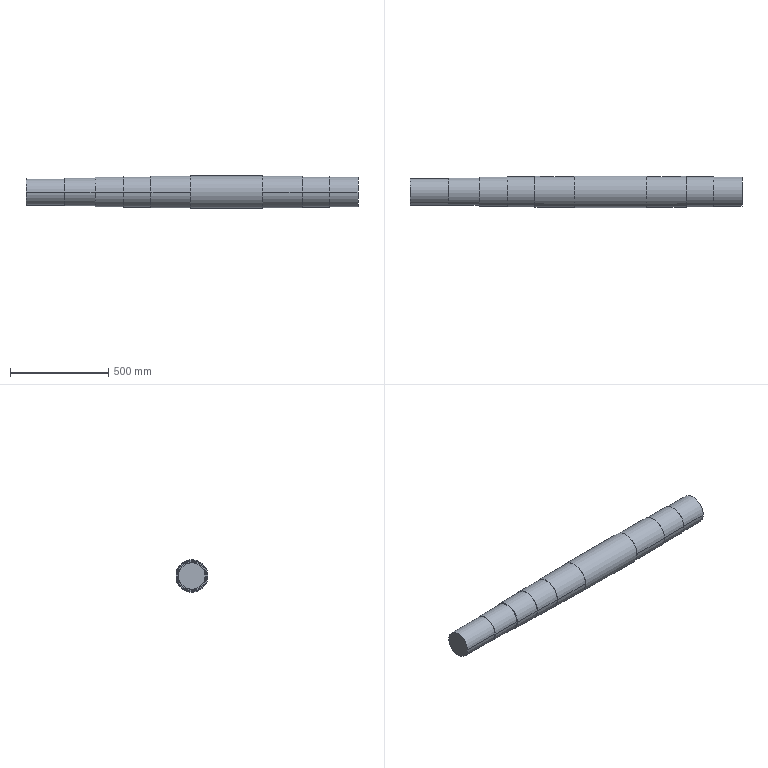Part | NX | features BREP 1 | 1 solid | 37 faces | box 1692 x 162.539 x 165 mm | volume 31180686 mm3 | cylinder 21 | plane 16 | commonest cylinder face diameters 150 x4 155 x4 160 x4 36 x2 40 x2 135 x2
STEP:
#1=CARTESIAN_POINT('',(-825.,70.,0.));
#2=VERTEX_POINT('',#1);
#3=CARTESIAN_POINT('',(-825.,-70.,0.));
#4=VERTEX_POINT('',#3);
#5=CARTESIAN_POINT('',(-825.,0.,0.));
#6=DIRECTION('',(1.,0.,0.));
#7=DIRECTION('',(0.,1.,0.));
#8=AXIS2_PLACEMENT_3D('',#5,#6,#7);
#9=CIRCLE('',#8,70.);
#10=EDGE_CURVE('',#2,#4,#9,.T.);
#11=ORIENTED_EDGE('',*,*,#10,.T.);
#12=CARTESIAN_POINT('',(-670.,-70.,0.));
#13=VERTEX_POINT('',#12);
#14=CARTESIAN_POINT('',(670.,-70.,0.));
#15=DIRECTION('',(1.,0.,0.));
#16=VECTOR('',#15,1000.);
#17=LINE('',#14,#16);
#18=EDGE_CURVE('',#4,#13,#17,.T.);
#19=ORIENTED_EDGE('',*,*,#18,.T.);
#20=CARTESIAN_POINT('',(-670.,70.,0.));
#21=VERTEX_POINT('',#20);
#22=CARTESIAN_POINT('',(-670.,0.,0.));
#23=DIRECTION('',(1.,0.,0.));
#24=DIRECTION('',(0.,1.,0.));
#25=AXIS2_PLACEMENT_3D('',#22,#23,#24);
#26=CIRCLE('',#25,70.);
#27=EDGE_CURVE('',#21,#13,#26,.T.);
#28=ORIENTED_EDGE('',*,*,#27,.F.);
#29=CARTESIAN_POINT('',(670.,70.,0.));
#30=DIRECTION('',(1.,0.,0.));
#31=VECTOR('',#30,1000.);
#32=LINE('',#29,#31);
#33=EDGE_CURVE('',#2,#21,#32,.T.);
#34=ORIENTED_EDGE('',*,*,#33,.F.);
#35=EDGE_LOOP('',(#11,#19,#28,#34));
#36=FACE_BOUND('',#35,.T.);
#37=CARTESIAN_POINT('',(670.,0.,0.));
#38=DIRECTION('',(1.,0.,0.));
#39=DIRECTION('',(0.,-1.,0.));
#40=AXIS2_PLACEMENT_3D('',#37,#38,#39);
#41=CYLINDRICAL_SURFACE('',#40,70.);
#42=ADVANCED_FACE('',(#36),#41,.T.);
#43=CARTESIAN_POINT('',(-670.,75.,0.));
#44=VERTEX_POINT('',#43);
#45=CARTESIAN_POINT('',(-670.,-75.,0.));
#46=VERTEX_POINT('',#45);
#47=CARTESIAN_POINT('',(-670.,0.,0.));
#48=DIRECTION('',(1.,0.,0.));
#49=DIRECTION('',(0.,1.,0.));
#50=AXIS2_PLACEMENT_3D('',#47,#48,#49);
#51=CIRCLE('',#50,75.);
#52=EDGE_CURVE('',#44,#46,#51,.T.);
#53=ORIENTED_EDGE('',*,*,#52,.T.);
#54=CARTESIAN_POINT('',(-527.,-75.,0.));
#55=VERTEX_POINT('',#54);
#56=CARTESIAN_POINT('',(670.,-75.,0.));
#57=DIRECTION('',(1.,0.,0.));
#58=VECTOR('',#57,1000.);
#59=LINE('',#56,#58);
#60=EDGE_CURVE('',#46,#55,#59,.T.);
#61=ORIENTED_EDGE('',*,*,#60,.T.);
#62=CARTESIAN_POINT('',(-527.,75.,0.));
#63=VERTEX_POINT('',#62);
#64=CARTESIAN_POINT('',(-527.,0.,0.));
#65=DIRECTION('',(1.,0.,0.));
#66=DIRECTION('',(0.,1.,0.));
#67=AXIS2_PLACEMENT_3D('',#64,#65,#66);
#68=CIRCLE('',#67,75.);
#69=EDGE_CURVE('',#63,#55,#68,.T.);
#70=ORIENTED_EDGE('',*,*,#69,.F.);
#71=CARTESIAN_POINT('',(670.,75.,0.));
#72=DIRECTION('',(1.,0.,0.));
#73=VECTOR('',#72,1000.);
#74=LINE('',#71,#73);
#75=EDGE_CURVE('',#44,#63,#74,.T.);
#76=ORIENTED_EDGE('',*,*,#75,.F.);
#77=EDGE_LOOP('',(#53,#61,#70,#76));
#78=FACE_BOUND('',#77,.T.);
#79=CARTESIAN_POINT('',(670.,0.,0.));
#80=DIRECTION('',(1.,0.,0.));
#81=DIRECTION('',(0.,-1.,0.));
#82=AXIS2_PLACEMENT_3D('',#79,#80,#81);
#83=CYLINDRICAL_SURFACE('',#82,75.);
#84=ADVANCED_FACE('',(#78),#83,.T.);
#85=CARTESIAN_POINT('',(-527.,77.5,0.));
#86=VERTEX_POINT('',#85);
#87=CARTESIAN_POINT('',(-527.,-77.5,0.));
#88=VERTEX_POINT('',#87);
#89=CARTESIAN_POINT('',(-527.,0.,0.));
#90=DIRECTION('',(1.,0.,0.));
#91=DIRECTION('',(0.,1.,0.));
#92=AXIS2_PLACEMENT_3D('',#89,#90,#91);
#93=CIRCLE('',#92,77.5);
#94=EDGE_CURVE('',#86,#88,#93,.T.);
#95=ORIENTED_EDGE('',*,*,#94,.T.);
#96=CARTESIAN_POINT('',(-385.,-77.5,0.));
#97=VERTEX_POINT('',#96);
#98=CARTESIAN_POINT('',(670.,-77.5,0.));
#99=DIRECTION('',(1.,0.,0.));
#100=VECTOR('',#99,1000.);
#101=LINE('',#98,#100);
#102=EDGE_CURVE('',#88,#97,#101,.T.);
#103=ORIENTED_EDGE('',*,*,#102,.T.);
#104=CARTESIAN_POINT('',(-385.,77.5,0.));
#105=VERTEX_POINT('',#104);
#106=CARTESIAN_POINT('',(-385.,0.,0.));
#107=DIRECTION('',(1.,0.,0.));
#108=DIRECTION('',(0.,1.,0.));
#109=AXIS2_PLACEMENT_3D('',#106,#107,#108);
#110=CIRCLE('',#109,77.5);
#111=EDGE_CURVE('',#105,#97,#110,.T.);
#112=ORIENTED_EDGE('',*,*,#111,.F.);
#113=CARTESIAN_POINT('',(670.,77.5,0.));
#114=DIRECTION('',(1.,0.,0.));
#115=VECTOR('',#114,1000.);
#116=LINE('',#113,#115);
#117=EDGE_CURVE('',#86,#105,#116,.T.);
#118=ORIENTED_EDGE('',*,*,#117,.F.);
#119=EDGE_LOOP('',(#95,#103,#112,#118));
#120=FACE_BOUND('',#119,.T.);
#121=CARTESIAN_POINT('',(670.,0.,0.));
#122=DIRECTION('',(1.,0.,0.));
#123=DIRECTION('',(0.,-1.,0.));
#124=AXIS2_PLACEMENT_3D('',#121,#122,#123);
#125=CYLINDRICAL_SURFACE('',#124,77.5);
#126=ADVANCED_FACE('',(#120),#125,.T.);
#127=CARTESIAN_POINT('',(385.,77.5,0.));
#128=VERTEX_POINT('',#127);
#129=CARTESIAN_POINT('',(385.,-77.5,0.));
#130=VERTEX_POINT('',#129);
#131=CARTESIAN_POINT('',(385.,0.,0.));
#132=DIRECTION('',(1.,0.,0.));
#133=DIRECTION('',(0.,1.,0.));
#134=AXIS2_PLACEMENT_3D('',#131,#132,#133);
#135=CIRCLE('',#134,77.5);
#136=EDGE_CURVE('',#128,#130,#135,.T.);
#137=ORIENTED_EDGE('',*,*,#136,.T.);
#138=CARTESIAN_POINT('',(527.,-77.5,0.));
#139=VERTEX_POINT('',#138);
#140=CARTESIAN_POINT('',(670.,-77.5,0.));
#141=DIRECTION('',(1.,0.,0.));
#142=VECTOR('',#141,1000.);
#143=LINE('',#140,#142);
#144=EDGE_CURVE('',#130,#139,#143,.T.);
#145=ORIENTED_EDGE('',*,*,#144,.T.);
#146=CARTESIAN_POINT('',(527.,77.5,0.));
#147=VERTEX_POINT('',#146);
#148=CARTESIAN_POINT('',(527.,0.,0.));
#149=DIRECTION('',(1.,0.,0.));
#150=DIRECTION('',(0.,1.,0.));
#151=AXIS2_PLACEMENT_3D('',#148,#149,#150);
#152=CIRCLE('',#151,77.5);
#153=EDGE_CURVE('',#147,#139,#152,.T.);
#154=ORIENTED_EDGE('',*,*,#153,.F.);
#155=CARTESIAN_POINT('',(670.,77.5,0.));
#156=DIRECTION('',(1.,0.,0.));
#157=VECTOR('',#156,1000.);
#158=LINE('',#155,#157);
#159=EDGE_CURVE('',#128,#147,#158,.T.);
#160=ORIENTED_EDGE('',*,*,#159,.F.);
#161=EDGE_LOOP('',(#137,#145,#154,#160));
#162=FACE_BOUND('',#161,.T.);
#163=CARTESIAN_POINT('',(670.,0.,0.));
#164=DIRECTION('',(1.,0.,0.));
#165=DIRECTION('',(0.,-1.,0.));
#166=AXIS2_PLACEMENT_3D('',#163,#164,#165);
#167=CYLINDRICAL_SURFACE('',#166,77.5);
#168=ADVANCED_FACE('',(#162),#167,.T.);
#169=CARTESIAN_POINT('',(527.,75.,0.));
#170=VERTEX_POINT('',#169);
#171=CARTESIAN_POINT('',(527.,-75.,0.));
#172=VERTEX_POINT('',#171);
#173=CARTESIAN_POINT('',(527.,0.,0.));
#174=DIRECTION('',(1.,0.,0.));
#175=DIRECTION('',(0.,1.,0.));
#176=AXIS2_PLACEMENT_3D('',#173,#174,#175);
#177=CIRCLE('',#176,75.);
#178=EDGE_CURVE('',#170,#172,#177,.T.);
#179=ORIENTED_EDGE('',*,*,#178,.T.);
#180=CARTESIAN_POINT('',(670.,-75.,0.));
#181=VERTEX_POINT('',#180);
#182=CARTESIAN_POINT('',(670.,-75.,0.));
#183=DIRECTION('',(1.,0.,0.));
#184=VECTOR('',#183,1000.);
#185=LINE('',#182,#184);
#186=EDGE_CURVE('',#172,#181,#185,.T.);
#187=ORIENTED_EDGE('',*,*,#186,.T.);
#188=CARTESIAN_POINT('',(670.,75.,0.));
#189=VERTEX_POINT('',#188);
#190=CARTESIAN_POINT('',(670.,0.,0.));
#191=DIRECTION('',(1.,0.,0.));
#192=DIRECTION('',(0.,1.,0.));
#193=AXIS2_PLACEMENT_3D('',#190,#191,#192);
#194=CIRCLE('',#193,75.);
#195=EDGE_CURVE('',#189,#181,#194,.T.);
#196=ORIENTED_EDGE('',*,*,#195,.F.);
#197=CARTESIAN_POINT('',(670.,75.,0.));
#198=DIRECTION('',(1.,0.,0.));
#199=VECTOR('',#198,1000.);
#200=LINE('',#197,#199);
#201=EDGE_CURVE('',#170,#189,#200,.T.);
#202=ORIENTED_EDGE('',*,*,#201,.F.);
#203=EDGE_LOOP('',(#179,#187,#196,#202));
#204=FACE_BOUND('',#203,.T.);
#205=CARTESIAN_POINT('',(670.,0.,0.));
#206=DIRECTION('',(1.,0.,0.));
#207=DIRECTION('',(0.,-1.,0.));
#208=AXIS2_PLACEMENT_3D('',#205,#206,#207);
#209=CYLINDRICAL_SURFACE('',#208,75.);
#210=ADVANCED_FACE('',(#204),#209,.T.);
#211=CARTESIAN_POINT('',(-385.,80.,0.));
#212=VERTEX_POINT('',#211);
#213=CARTESIAN_POINT('',(-385.,-80.,0.));
#214=VERTEX_POINT('',#213);
#215=CARTESIAN_POINT('',(-385.,0.,0.));
#216=DIRECTION('',(1.,0.,0.));
#217=DIRECTION('',(0.,1.,0.));
#218=AXIS2_PLACEMENT_3D('',#215,#216,#217);
#219=CIRCLE('',#218,80.);
#220=EDGE_CURVE('',#212,#214,#219,.T.);
#221=ORIENTED_EDGE('',*,*,#220,.T.);
#222=CARTESIAN_POINT('',(-185.,-80.,0.));
#223=VERTEX_POINT('',#222);
#224=CARTESIAN_POINT('',(670.,-80.,0.));
#225=DIRECTION('',(1.,0.,0.));
#226=VECTOR('',#225,1000.);
#227=LINE('',#224,#226);
#228=EDGE_CURVE('',#214,#223,#227,.T.);
#229=ORIENTED_EDGE('',*,*,#228,.T.);
#230=CARTESIAN_POINT('',(-185.,77.46,20.));
#231=VERTEX_POINT('',#230);
#232=CARTESIAN_POINT('',(-185.,0.,0.));
#233=DIRECTION('',(1.,0.,0.));
#234=DIRECTION('',(0.,1.,0.));
#235=AXIS2_PLACEMENT_3D('',#232,#233,#234);
#236=CIRCLE('',#235,80.);
#237=EDGE_CURVE('',#231,#223,#236,.T.);
#238=ORIENTED_EDGE('',*,*,#237,.F.);
#239=CARTESIAN_POINT('',(-350.,77.46,20.));
#240=VERTEX_POINT('',#239);
#241=CARTESIAN_POINT('',(670.,77.46,20.));
#242=DIRECTION('',(-1.,0.,0.));
#243=VECTOR('',#242,1000.);
#244=LINE('',#241,#243);
#245=EDGE_CURVE('',#231,#240,#244,.T.);
#246=ORIENTED_EDGE('',*,*,#245,.T.);
#247=CARTESIAN_POINT('',(-370.,80.,0.));
#248=VERTEX_POINT('',#247);
#249=CARTESIAN_POINT('',(-350.,77.46,20.));
#250=CARTESIAN_POINT('',(-352.652,77.46,20.));
#251=CARTESIAN_POINT('',(-357.872,77.743,18.946));
#252=CARTESIAN_POINT('',(-364.505,78.742,14.509));
#253=CARTESIAN_POINT('',(-368.936,79.725,7.897));
#254=CARTESIAN_POINT('',(-370.,80.,2.652));
#255=CARTESIAN_POINT('',(-370.,80.,0.));
#256=B_SPLINE_CURVE_WITH_KNOTS('',3,(#249,#250,#251,#252,#253,#254,#255),.UNSPECIFIED.,.F.,.F.,(4,1,1,1,4),(0.,0.007842,0.01568,0.02353,0.03137),.UNSPECIFIED.);
#257=EDGE_CURVE('',#240,#248,#256,.T.);
#258=ORIENTED_EDGE('',*,*,#257,.T.);
#259=CARTESIAN_POINT('',(670.,80.,0.));
#260=DIRECTION('',(1.,0.,0.));
#261=VECTOR('',#260,1000.);
#262=LINE('',#259,#261);
#263=EDGE_CURVE('',#212,#248,#262,.T.);
#264=ORIENTED_EDGE('',*,*,#263,.F.);
#265=EDGE_LOOP('',(#221,#229,#238,#246,#258,#264));
#266=FACE_BOUND('',#265,.T.);
#267=CARTESIAN_POINT('',(670.,0.,0.));
#268=DIRECTION('',(1.,0.,0.));
#269=DIRECTION('',(0.,-1.,0.));
#270=AXIS2_PLACEMENT_3D('',#267,#268,#269);
#271=CYLINDRICAL_SURFACE('',#270,80.);
#272=ADVANCED_FACE('',(#266),#271,.T.);
#273=CARTESIAN_POINT('',(185.,77.46,20.));
#274=VERTEX_POINT('',#273);
#275=CARTESIAN_POINT('',(185.,-80.,0.));
#276=VERTEX_POINT('',#275);
#277=CARTESIAN_POINT('',(185.,0.,0.));
#278=DIRECTION('',(1.,0.,0.));
#279=DIRECTION('',(0.,1.,0.));
#280=AXIS2_PLACEMENT_3D('',#277,#278,#279);
#281=CIRCLE('',#280,80.);
#282=EDGE_CURVE('',#274,#276,#281,.T.);
#283=ORIENTED_EDGE('',*,*,#282,.T.);
#284=CARTESIAN_POINT('',(385.,-80.,0.));
#285=VERTEX_POINT('',#284);
#286=CARTESIAN_POINT('',(670.,-80.,0.));
#287=DIRECTION('',(1.,0.,0.));
#288=VECTOR('',#287,1000.);
#289=LINE('',#286,#288);
#290=EDGE_CURVE('',#276,#285,#289,.T.);
#291=ORIENTED_EDGE('',*,*,#290,.T.);
#292=CARTESIAN_POINT('',(385.,80.,0.));
#293=VERTEX_POINT('',#292);
#294=CARTESIAN_POINT('',(385.,0.,0.));
#295=DIRECTION('',(1.,0.,0.));
#296=DIRECTION('',(0.,1.,0.));
#297=AXIS2_PLACEMENT_3D('',#294,#295,#296);
#298=CIRCLE('',#297,80.);
#299=EDGE_CURVE('',#293,#285,#298,.T.);
#300=ORIENTED_EDGE('',*,*,#299,.F.);
#301=CARTESIAN_POINT('',(370.,80.,0.));
#302=VERTEX_POINT('',#301);
#303=CARTESIAN_POINT('',(670.,80.,0.));
#304=DIRECTION('',(1.,0.,0.));
#305=VECTOR('',#304,1000.);
#306=LINE('',#303,#305);
#307=EDGE_CURVE('',#302,#293,#306,.T.);
#308=ORIENTED_EDGE('',*,*,#307,.F.);
#309=CARTESIAN_POINT('',(350.,77.46,20.));
#310=VERTEX_POINT('',#309);
#311=CARTESIAN_POINT('',(370.,80.,0.));
#312=CARTESIAN_POINT('',(370.,80.,2.652));
#313=CARTESIAN_POINT('',(368.946,79.727,7.872));
#314=CARTESIAN_POINT('',(364.507,78.743,14.507));
#315=CARTESIAN_POINT('',(357.897,77.745,18.936));
#316=CARTESIAN_POINT('',(352.652,77.46,20.));
#317=CARTESIAN_POINT('',(350.,77.46,20.));
#318=B_SPLINE_CURVE_WITH_KNOTS('',3,(#311,#312,#313,#314,#315,#316,#317),.UNSPECIFIED.,.F.,.F.,(4,1,1,1,4),(0.,0.007842,0.01568,0.02353,0.03137),.UNSPECIFIED.);
#319=EDGE_CURVE('',#302,#310,#318,.T.);
#320=ORIENTED_EDGE('',*,*,#319,.T.);
#321=CARTESIAN_POINT('',(670.,77.46,20.));
#322=DIRECTION('',(-1.,0.,0.));
#323=VECTOR('',#322,1000.);
#324=LINE('',#321,#323);
#325=EDGE_CURVE('',#310,#274,#324,.T.);
#326=ORIENTED_EDGE('',*,*,#325,.T.);
#327=EDGE_LOOP('',(#283,#291,#300,#308,#320,#326));
#328=FACE_BOUND('',#327,.T.);
#329=CARTESIAN_POINT('',(670.,0.,0.));
#330=DIRECTION('',(1.,0.,0.));
#331=DIRECTION('',(0.,-1.,0.));
#332=AXIS2_PLACEMENT_3D('',#329,#330,#331);
#333=CYLINDRICAL_SURFACE('',#332,80.);
#334=ADVANCED_FACE('',(#328),#333,.T.);
#335=CARTESIAN_POINT('',(-1022.,67.5,0.));
#336=VERTEX_POINT('',#335);
#337=CARTESIAN_POINT('',(-1022.,-67.5,0.));
#338=VERTEX_POINT('',#337);
#339=CARTESIAN_POINT('',(-1022.,0.,0.));
#340=DIRECTION('',(1.,0.,0.));
#341=DIRECTION('',(0.,1.,0.));
#342=AXIS2_PLACEMENT_3D('',#339,#340,#341);
#343=CIRCLE('',#342,67.5);
#344=EDGE_CURVE('',#336,#338,#343,.T.);
#345=ORIENTED_EDGE('',*,*,#344,.T.);
#346=CARTESIAN_POINT('',(-825.,-67.5,0.));
#347=VERTEX_POINT('',#346);
#348=CARTESIAN_POINT('',(670.,-67.5,0.));
#349=DIRECTION('',(1.,0.,0.));
#350=VECTOR('',#349,1000.);
#351=LINE('',#348,#350);
#352=EDGE_CURVE('',#338,#347,#351,.T.);
#353=ORIENTED_EDGE('',*,*,#352,.T.);
#354=CARTESIAN_POINT('',(-825.,67.5,0.));
#355=VERTEX_POINT('',#354);
#356=CARTESIAN_POINT('',(-825.,0.,0.));
#357=DIRECTION('',(1.,0.,0.));
#358=DIRECTION('',(0.,1.,0.));
#359=AXIS2_PLACEMENT_3D('',#356,#357,#358);
#360=CIRCLE('',#359,67.5);
#361=EDGE_CURVE('',#355,#347,#360,.T.);
#362=ORIENTED_EDGE('',*,*,#361,.F.);
#363=CARTESIAN_POINT('',(-832.,67.5,0.));
#364=VERTEX_POINT('',#363);
#365=CARTESIAN_POINT('',(670.,67.5,0.));
#366=DIRECTION('',(1.,0.,0.));
#367=VECTOR('',#366,1000.);
#368=LINE('',#365,#367);
#369=EDGE_CURVE('',#364,#355,#368,.T.);
#370=ORIENTED_EDGE('',*,*,#369,.F.);
#371=CARTESIAN_POINT('',(-850.,65.056,18.));
#372=VERTEX_POINT('',#371);
#373=CARTESIAN_POINT('',(-832.,67.5,0.));
#374=CARTESIAN_POINT('',(-832.,67.5,2.389));
#375=CARTESIAN_POINT('',(-832.95,67.238,7.089));
#376=CARTESIAN_POINT('',(-836.944,66.292,13.056));
#377=CARTESIAN_POINT('',(-842.89,65.332,17.041));
#378=CARTESIAN_POINT('',(-847.611,65.056,18.));
#379=CARTESIAN_POINT('',(-850.,65.056,18.));
#380=B_SPLINE_CURVE_WITH_KNOTS('',3,(#373,#374,#375,#376,#377,#378,#379),.UNSPECIFIED.,.F.,.F.,(4,1,1,1,4),(0.,0.007062,0.01412,0.02119,0.02825),.UNSPECIFIED.);
#381=EDGE_CURVE('',#364,#372,#380,.T.);
#382=ORIENTED_EDGE('',*,*,#381,.T.);
#383=CARTESIAN_POINT('',(-994.,65.056,18.));
#384=VERTEX_POINT('',#383);
#385=CARTESIAN_POINT('',(670.,65.056,18.));
#386=DIRECTION('',(-1.,0.,0.));
#387=VECTOR('',#386,1000.);
#388=LINE('',#385,#387);
#389=EDGE_CURVE('',#372,#384,#388,.T.);
#390=ORIENTED_EDGE('',*,*,#389,.T.);
#391=CARTESIAN_POINT('',(-1012.,67.5,0.));
#392=VERTEX_POINT('',#391);
#393=CARTESIAN_POINT('',(-994.,65.056,18.));
#394=CARTESIAN_POINT('',(-996.389,65.056,18.));
#395=CARTESIAN_POINT('',(-1001.088,65.33,17.05));
#396=CARTESIAN_POINT('',(-1007.054,66.291,13.058));
#397=CARTESIAN_POINT('',(-1011.041,67.235,7.111));
#398=CARTESIAN_POINT('',(-1012.,67.5,2.389));
#399=CARTESIAN_POINT('',(-1012.,67.5,0.));
#400=B_SPLINE_CURVE_WITH_KNOTS('',3,(#393,#394,#395,#396,#397,#398,#399),.UNSPECIFIED.,.F.,.F.,(4,1,1,1,4),(0.,0.007062,0.01412,0.02119,0.02825),.UNSPECIFIED.);
#401=EDGE_CURVE('',#384,#392,#400,.T.);
#402=ORIENTED_EDGE('',*,*,#401,.T.);
#403=CARTESIAN_POINT('',(670.,67.5,0.));
#404=DIRECTION('',(1.,0.,0.));
#405=VECTOR('',#404,1000.);
#406=LINE('',#403,#405);
#407=EDGE_CURVE('',#336,#392,#406,.T.);
#408=ORIENTED_EDGE('',*,*,#407,.F.);
#409=EDGE_LOOP('',(#345,#353,#362,#370,#382,#390,#402,#408));
#410=FACE_BOUND('',#409,.T.);
#411=CARTESIAN_POINT('',(670.,0.,0.));
#412=DIRECTION('',(1.,0.,0.));
#413=DIRECTION('',(0.,-1.,0.));
#414=AXIS2_PLACEMENT_3D('',#411,#412,#413);
#415=CYLINDRICAL_SURFACE('',#414,67.5);
#416=ADVANCED_FACE('',(#410),#415,.T.);
#417=ORIENTED_EDGE('',*,*,#352,.F.);
#418=CARTESIAN_POINT('',(-1022.,0.,0.));
#419=DIRECTION('',(1.,0.,0.));
#420=DIRECTION('',(0.,1.,0.));
#421=AXIS2_PLACEMENT_3D('',#418,#419,#420);
#422=CIRCLE('',#421,67.5);
#423=EDGE_CURVE('',#338,#336,#422,.T.);
#424=ORIENTED_EDGE('',*,*,#423,.T.);
#425=ORIENTED_EDGE('',*,*,#407,.T.);
#426=CARTESIAN_POINT('',(-994.,65.056,-18.));
#427=VERTEX_POINT('',#426);
#428=CARTESIAN_POINT('',(-1012.,67.5,0.));
#429=CARTESIAN_POINT('',(-1012.,67.5,-2.389));
#430=CARTESIAN_POINT('',(-1011.05,67.238,-7.089));
#431=CARTESIAN_POINT('',(-1007.056,66.292,-13.056));
#432=CARTESIAN_POINT('',(-1001.11,65.332,-17.041));
#433=CARTESIAN_POINT('',(-996.389,65.056,-18.));
#434=CARTESIAN_POINT('',(-994.,65.056,-18.));
#435=B_SPLINE_CURVE_WITH_KNOTS('',3,(#428,#429,#430,#431,#432,#433,#434),.UNSPECIFIED.,.F.,.F.,(4,1,1,1,4),(0.,0.007062,0.01412,0.02119,0.02825),.UNSPECIFIED.);
#436=EDGE_CURVE('',#392,#427,#435,.T.);
#437=ORIENTED_EDGE('',*,*,#436,.T.);
#438=CARTESIAN_POINT('',(-850.,65.056,-18.));
#439=VERTEX_POINT('',#438);
#440=CARTESIAN_POINT('',(670.,65.056,-18.));
#441=DIRECTION('',(1.,0.,0.));
#442=VECTOR('',#441,1000.);
#443=LINE('',#440,#442);
#444=EDGE_CURVE('',#427,#439,#443,.T.);
#445=ORIENTED_EDGE('',*,*,#444,.T.);
#446=CARTESIAN_POINT('',(-850.,65.056,-18.));
#447=CARTESIAN_POINT('',(-847.611,65.056,-18.));
#448=CARTESIAN_POINT('',(-842.912,65.33,-17.05));
#449=CARTESIAN_POINT('',(-836.946,66.291,-13.058));
#450=CARTESIAN_POINT('',(-832.959,67.235,-7.111));
#451=CARTESIAN_POINT('',(-832.,67.5,-2.389));
#452=CARTESIAN_POINT('',(-832.,67.5,0.));
#453=B_SPLINE_CURVE_WITH_KNOTS('',3,(#446,#447,#448,#449,#450,#451,#452),.UNSPECIFIED.,.F.,.F.,(4,1,1,1,4),(0.,0.007062,0.01412,0.02119,0.02825),.UNSPECIFIED.);
#454=EDGE_CURVE('',#439,#364,#453,.T.);
#455=ORIENTED_EDGE('',*,*,#454,.T.);
#456=ORIENTED_EDGE('',*,*,#369,.T.);
#457=CARTESIAN_POINT('',(-825.,0.,0.));
#458=DIRECTION('',(1.,0.,0.));
#459=DIRECTION('',(0.,1.,0.));
#460=AXIS2_PLACEMENT_3D('',#457,#458,#459);
#461=CIRCLE('',#460,67.5);
#462=EDGE_CURVE('',#347,#355,#461,.T.);
#463=ORIENTED_EDGE('',*,*,#462,.F.);
#464=EDGE_LOOP('',(#417,#424,#425,#437,#445,#455,#456,#463));
#465=FACE_BOUND('',#464,.T.);
#466=CARTESIAN_POINT('',(670.,0.,0.));
#467=DIRECTION('',(1.,0.,0.));
#468=DIRECTION('',(0.,-1.,0.));
#469=AXIS2_PLACEMENT_3D('',#466,#467,#468);
#470=CYLINDRICAL_SURFACE('',#469,67.5);
#471=ADVANCED_FACE('',(#465),#470,.T.);
#472=ORIENTED_EDGE('',*,*,#290,.F.);
#473=CARTESIAN_POINT('',(185.,77.46,-20.));
#474=VERTEX_POINT('',#473);
#475=CARTESIAN_POINT('',(185.,0.,0.));
#476=DIRECTION('',(1.,0.,0.));
#477=DIRECTION('',(0.,1.,0.));
#478=AXIS2_PLACEMENT_3D('',#475,#476,#477);
#479=CIRCLE('',#478,80.);
#480=EDGE_CURVE('',#276,#474,#479,.T.);
#481=ORIENTED_EDGE('',*,*,#480,.T.);
#482=CARTESIAN_POINT('',(350.,77.46,-20.));
#483=VERTEX_POINT('',#482);
#484=CARTESIAN_POINT('',(670.,77.46,-20.));
#485=DIRECTION('',(1.,0.,0.));
#486=VECTOR('',#485,1000.);
#487=LINE('',#484,#486);
#488=EDGE_CURVE('',#474,#483,#487,.T.);
#489=ORIENTED_EDGE('',*,*,#488,.T.);
#490=CARTESIAN_POINT('',(350.,77.46,-20.));
#491=CARTESIAN_POINT('',(352.652,77.46,-20.));
#492=CARTESIAN_POINT('',(357.872,77.743,-18.946));
#493=CARTESIAN_POINT('',(364.505,78.742,-14.509));
#494=CARTESIAN_POINT('',(368.936,79.725,-7.897));
#495=CARTESIAN_POINT('',(370.,80.,-2.652));
#496=CARTESIAN_POINT('',(370.,80.,0.));
#497=B_SPLINE_CURVE_WITH_KNOTS('',3,(#490,#491,#492,#493,#494,#495,#496),.UNSPECIFIED.,.F.,.F.,(4,1,1,1,4),(0.,0.007842,0.01568,0.02353,0.03137),.UNSPECIFIED.);
#498=EDGE_CURVE('',#483,#302,#497,.T.);
#499=ORIENTED_EDGE('',*,*,#498,.T.);
#500=ORIENTED_EDGE('',*,*,#307,.T.);
#501=CARTESIAN_POINT('',(385.,0.,0.));
#502=DIRECTION('',(1.,0.,0.));
#503=DIRECTION('',(0.,1.,0.));
#504=AXIS2_PLACEMENT_3D('',#501,#502,#503);
#505=CIRCLE('',#504,80.);
#506=EDGE_CURVE('',#285,#293,#505,.T.);
#507=ORIENTED_EDGE('',*,*,#506,.F.);
#508=EDGE_LOOP('',(#472,#481,#489,#499,#500,#507));
#509=FACE_BOUND('',#508,.T.);
#510=CARTESIAN_POINT('',(670.,0.,0.));
#511=DIRECTION('',(1.,0.,0.));
#512=DIRECTION('',(0.,-1.,0.));
#513=AXIS2_PLACEMENT_3D('',#510,#511,#512);
#514=CYLINDRICAL_SURFACE('',#513,80.);
#515=ADVANCED_FACE('',(#509),#514,.T.);
#516=ORIENTED_EDGE('',*,*,#282,.F.);
#517=CARTESIAN_POINT('',(185.,80.039,20.));
#518=VERTEX_POINT('',#517);
#519=CARTESIAN_POINT('',(185.,82.5,20.));
#520=DIRECTION('',(0.,1.,0.));
#521=VECTOR('',#520,1000.);
#522=LINE('',#519,#521);
#523=EDGE_CURVE('',#274,#518,#522,.T.);
#524=ORIENTED_EDGE('',*,*,#523,.T.);
#525=CARTESIAN_POINT('',(185.,80.039,-20.));
#526=VERTEX_POINT('',#525);
#527=CARTESIAN_POINT('',(185.,0.,0.));
#528=DIRECTION('',(1.,0.,0.));
#529=DIRECTION('',(0.,1.,0.));
#530=AXIS2_PLACEMENT_3D('',#527,#528,#529);
#531=CIRCLE('',#530,82.5);
#532=EDGE_CURVE('',#518,#526,#531,.T.);
#533=ORIENTED_EDGE('',*,*,#532,.T.);
#534=CARTESIAN_POINT('',(185.,82.5,-20.));
#535=DIRECTION('',(0.,-1.,0.));
#536=VECTOR('',#535,1000.);
#537=LINE('',#534,#536);
#538=EDGE_CURVE('',#526,#474,#537,.T.);
#539=ORIENTED_EDGE('',*,*,#538,.T.);
#540=ORIENTED_EDGE('',*,*,#480,.F.);
#541=EDGE_LOOP('',(#516,#524,#533,#539,#540));
#542=FACE_BOUND('',#541,.T.);
#543=CARTESIAN_POINT('',(185.,82.5,0.));
#544=DIRECTION('',(1.,0.,0.));
#545=DIRECTION('',(0.,-1.,0.));
#546=AXIS2_PLACEMENT_3D('',#543,#544,#545);
#547=PLANE('',#546);
#548=ADVANCED_FACE('',(#542),#547,.T.);
#549=ORIENTED_EDGE('',*,*,#532,.F.);
#550=CARTESIAN_POINT('',(-185.,80.039,20.));
#551=VERTEX_POINT('',#550);
#552=CARTESIAN_POINT('',(670.,80.039,20.));
#553=DIRECTION('',(-1.,0.,0.));
#554=VECTOR('',#553,1000.);
#555=LINE('',#552,#554);
#556=EDGE_CURVE('',#518,#551,#555,.T.);
#557=ORIENTED_EDGE('',*,*,#556,.T.);
#558=CARTESIAN_POINT('',(-185.,80.039,-20.));
#559=VERTEX_POINT('',#558);
#560=CARTESIAN_POINT('',(-185.,0.,0.));
#561=DIRECTION('',(1.,0.,0.));
#562=DIRECTION('',(0.,1.,0.));
#563=AXIS2_PLACEMENT_3D('',#560,#561,#562);
#564=CIRCLE('',#563,82.5);
#565=EDGE_CURVE('',#551,#559,#564,.T.);
#566=ORIENTED_EDGE('',*,*,#565,.T.);
#567=CARTESIAN_POINT('',(670.,80.039,-20.));
#568=DIRECTION('',(1.,0.,0.));
#569=VECTOR('',#568,1000.);
#570=LINE('',#567,#569);
#571=EDGE_CURVE('',#559,#526,#570,.T.);
#572=ORIENTED_EDGE('',*,*,#571,.T.);
#573=EDGE_LOOP('',(#549,#557,#566,#572));
#574=FACE_BOUND('',#573,.T.);
#575=CARTESIAN_POINT('',(670.,0.,0.));
#576=DIRECTION('',(1.,0.,0.));
#577=DIRECTION('',(0.,-1.,0.));
#578=AXIS2_PLACEMENT_3D('',#575,#576,#577);
#579=CYLINDRICAL_SURFACE('',#578,82.5);
#580=ADVANCED_FACE('',(#574),#579,.T.);
#581=ORIENTED_EDGE('',*,*,#565,.F.);
#582=CARTESIAN_POINT('',(-185.,82.5,20.));
#583=DIRECTION('',(0.,-1.,0.));
#584=VECTOR('',#583,1000.);
#585=LINE('',#582,#584);
#586=EDGE_CURVE('',#551,#231,#585,.T.);
#587=ORIENTED_EDGE('',*,*,#586,.T.);
#588=ORIENTED_EDGE('',*,*,#237,.T.);
#589=CARTESIAN_POINT('',(-185.,77.46,-20.));
#590=VERTEX_POINT('',#589);
#591=CARTESIAN_POINT('',(-185.,0.,0.));
#592=DIRECTION('',(1.,0.,0.));
#593=DIRECTION('',(0.,1.,0.));
#594=AXIS2_PLACEMENT_3D('',#591,#592,#593);
#595=CIRCLE('',#594,80.);
#596=EDGE_CURVE('',#223,#590,#595,.T.);
#597=ORIENTED_EDGE('',*,*,#596,.T.);
#598=CARTESIAN_POINT('',(-185.,82.5,-20.));
#599=DIRECTION('',(0.,1.,0.));
#600=VECTOR('',#599,1000.);
#601=LINE('',#598,#600);
#602=EDGE_CURVE('',#590,#559,#601,.T.);
#603=ORIENTED_EDGE('',*,*,#602,.T.);
#604=EDGE_LOOP('',(#581,#587,#588,#597,#603));
#605=FACE_BOUND('',#604,.T.);
#606=CARTESIAN_POINT('',(-185.,82.5,0.));
#607=DIRECTION('',(-1.,0.,0.));
#608=DIRECTION('',(0.,1.,0.));
#609=AXIS2_PLACEMENT_3D('',#606,#607,#608);
#610=PLANE('',#609);
#611=ADVANCED_FACE('',(#605),#610,.T.);
#612=ORIENTED_EDGE('',*,*,#228,.F.);
#613=CARTESIAN_POINT('',(-385.,0.,0.));
#614=DIRECTION('',(1.,0.,0.));
#615=DIRECTION('',(0.,1.,0.));
#616=AXIS2_PLACEMENT_3D('',#613,#614,#615);
#617=CIRCLE('',#616,80.);
#618=EDGE_CURVE('',#214,#212,#617,.T.);
#619=ORIENTED_EDGE('',*,*,#618,.T.);
#620=ORIENTED_EDGE('',*,*,#263,.T.);
#621=CARTESIAN_POINT('',(-350.,77.46,-20.));
#622=VERTEX_POINT('',#621);
#623=CARTESIAN_POINT('',(-370.,80.,0.));
#624=CARTESIAN_POINT('',(-370.,80.,-2.652));
#625=CARTESIAN_POINT('',(-368.946,79.727,-7.872));
#626=CARTESIAN_POINT('',(-364.507,78.743,-14.507));
#627=CARTESIAN_POINT('',(-357.897,77.745,-18.936));
#628=CARTESIAN_POINT('',(-352.652,77.46,-20.));
#629=CARTESIAN_POINT('',(-350.,77.46,-20.));
#630=B_SPLINE_CURVE_WITH_KNOTS('',3,(#623,#624,#625,#626,#627,#628,#629),.UNSPECIFIED.,.F.,.F.,(4,1,1,1,4),(0.,0.007842,0.01568,0.02353,0.03137),.UNSPECIFIED.);
#631=EDGE_CURVE('',#248,#622,#630,.T.);
#632=ORIENTED_EDGE('',*,*,#631,.T.);
#633=CARTESIAN_POINT('',(670.,77.46,-20.));
#634=DIRECTION('',(1.,0.,0.));
#635=VECTOR('',#634,1000.);
#636=LINE('',#633,#635);
#637=EDGE_CURVE('',#622,#590,#636,.T.);
#638=ORIENTED_EDGE('',*,*,#637,.T.);
#639=ORIENTED_EDGE('',*,*,#596,.F.);
#640=EDGE_LOOP('',(#612,#619,#620,#632,#638,#639));
#641=FACE_BOUND('',#640,.T.);
#642=CARTESIAN_POINT('',(670.,0.,0.));
#643=DIRECTION('',(1.,0.,0.));
#644=DIRECTION('',(0.,-1.,0.));
#645=AXIS2_PLACEMENT_3D('',#642,#643,#644);
#646=CYLINDRICAL_SURFACE('',#645,80.);
#647=ADVANCED_FACE('',(#641),#646,.T.);
#648=ORIENTED_EDGE('',*,*,#195,.T.);
#649=CARTESIAN_POINT('',(670.,0.,0.));
#650=DIRECTION('',(1.,0.,0.));
#651=DIRECTION('',(0.,1.,0.));
#652=AXIS2_PLACEMENT_3D('',#649,#650,#651);
#653=CIRCLE('',#652,75.);
#654=EDGE_CURVE('',#181,#189,#653,.T.);
#655=ORIENTED_EDGE('',*,*,#654,.T.);
#656=EDGE_LOOP('',(#648,#655));
#657=FACE_BOUND('',#656,.T.);
#658=CARTESIAN_POINT('',(670.,75.,0.));
#659=DIRECTION('',(1.,0.,0.));
#660=DIRECTION('',(0.,-1.,0.));
#661=AXIS2_PLACEMENT_3D('',#658,#659,#660);
#662=PLANE('',#661);
#663=ADVANCED_FACE('',(#657),#662,.T.);
#664=ORIENTED_EDGE('',*,*,#186,.F.);
#665=CARTESIAN_POINT('',(527.,0.,0.));
#666=DIRECTION('',(1.,0.,0.));
#667=DIRECTION('',(0.,1.,0.));
#668=AXIS2_PLACEMENT_3D('',#665,#666,#667);
#669=CIRCLE('',#668,75.);
#670=EDGE_CURVE('',#172,#170,#669,.T.);
#671=ORIENTED_EDGE('',*,*,#670,.T.);
#672=ORIENTED_EDGE('',*,*,#201,.T.);
#673=ORIENTED_EDGE('',*,*,#654,.F.);
#674=EDGE_LOOP('',(#664,#671,#672,#673));
#675=FACE_BOUND('',#674,.T.);
#676=CARTESIAN_POINT('',(670.,0.,0.));
#677=DIRECTION('',(1.,0.,0.));
#678=DIRECTION('',(0.,-1.,0.));
#679=AXIS2_PLACEMENT_3D('',#676,#677,#678);
#680=CYLINDRICAL_SURFACE('',#679,75.);
#681=ADVANCED_FACE('',(#675),#680,.T.);
#682=ORIENTED_EDGE('',*,*,#153,.T.);
#683=CARTESIAN_POINT('',(527.,0.,0.));
#684=DIRECTION('',(1.,0.,0.));
#685=DIRECTION('',(0.,1.,0.));
#686=AXIS2_PLACEMENT_3D('',#683,#684,#685);
#687=CIRCLE('',#686,77.5);
#688=EDGE_CURVE('',#139,#147,#687,.T.);
#689=ORIENTED_EDGE('',*,*,#688,.T.);
#690=EDGE_LOOP('',(#682,#689));
#691=FACE_BOUND('',#690,.T.);
#692=ORIENTED_EDGE('',*,*,#178,.F.);
#693=ORIENTED_EDGE('',*,*,#670,.F.);
#694=EDGE_LOOP('',(#692,#693));
#695=FACE_BOUND('',#694,.T.);
#696=CARTESIAN_POINT('',(527.,77.5,0.));
#697=DIRECTION('',(1.,0.,0.));
#698=DIRECTION('',(0.,-1.,0.));
#699=AXIS2_PLACEMENT_3D('',#696,#697,#698);
#700=PLANE('',#699);
#701=ADVANCED_FACE('',(#691,#695),#700,.T.);
#702=ORIENTED_EDGE('',*,*,#144,.F.);
#703=CARTESIAN_POINT('',(385.,0.,0.));
#704=DIRECTION('',(1.,0.,0.));
#705=DIRECTION('',(0.,1.,0.));
#706=AXIS2_PLACEMENT_3D('',#703,#704,#705);
#707=CIRCLE('',#706,77.5);
#708=EDGE_CURVE('',#130,#128,#707,.T.);
#709=ORIENTED_EDGE('',*,*,#708,.T.);
#710=ORIENTED_EDGE('',*,*,#159,.T.);
#711=ORIENTED_EDGE('',*,*,#688,.F.);
#712=EDGE_LOOP('',(#702,#709,#710,#711));
#713=FACE_BOUND('',#712,.T.);
#714=CARTESIAN_POINT('',(670.,0.,0.));
#715=DIRECTION('',(1.,0.,0.));
#716=DIRECTION('',(0.,-1.,0.));
#717=AXIS2_PLACEMENT_3D('',#714,#715,#716);
#718=CYLINDRICAL_SURFACE('',#717,77.5);
#719=ADVANCED_FACE('',(#713),#718,.T.);
#720=ORIENTED_EDGE('',*,*,#299,.T.);
#721=ORIENTED_EDGE('',*,*,#506,.T.);
#722=EDGE_LOOP('',(#720,#721));
#723=FACE_BOUND('',#722,.T.);
#724=ORIENTED_EDGE('',*,*,#136,.F.);
#725=ORIENTED_EDGE('',*,*,#708,.F.);
#726=EDGE_LOOP('',(#724,#725));
#727=FACE_BOUND('',#726,.T.);
#728=CARTESIAN_POINT('',(385.,80.,0.));
#729=DIRECTION('',(1.,0.,0.));
#730=DIRECTION('',(0.,-1.,0.));
#731=AXIS2_PLACEMENT_3D('',#728,#729,#730);
#732=PLANE('',#731);
#733=ADVANCED_FACE('',(#723,#727),#732,.T.);
#734=ORIENTED_EDGE('',*,*,#111,.T.);
#735=CARTESIAN_POINT('',(-385.,0.,0.));
#736=DIRECTION('',(1.,0.,0.));
#737=DIRECTION('',(0.,1.,0.));
#738=AXIS2_PLACEMENT_3D('',#735,#736,#737);
#739=CIRCLE('',#738,77.5);
#740=EDGE_CURVE('',#97,#105,#739,.T.);
#741=ORIENTED_EDGE('',*,*,#740,.T.);
#742=EDGE_LOOP('',(#734,#741));
#743=FACE_BOUND('',#742,.T.);
#744=ORIENTED_EDGE('',*,*,#220,.F.);
#745=ORIENTED_EDGE('',*,*,#618,.F.);
#746=EDGE_LOOP('',(#744,#745));
#747=FACE_BOUND('',#746,.T.);
#748=CARTESIAN_POINT('',(-385.,80.,0.));
#749=DIRECTION('',(-1.,0.,0.));
#750=DIRECTION('',(0.,1.,0.));
#751=AXIS2_PLACEMENT_3D('',#748,#749,#750);
#752=PLANE('',#751);
#753=ADVANCED_FACE('',(#743,#747),#752,.T.);
#754=ORIENTED_EDGE('',*,*,#102,.F.);
#755=CARTESIAN_POINT('',(-527.,0.,0.));
#756=DIRECTION('',(1.,0.,0.));
#757=DIRECTION('',(0.,1.,0.));
#758=AXIS2_PLACEMENT_3D('',#755,#756,#757);
#759=CIRCLE('',#758,77.5);
#760=EDGE_CURVE('',#88,#86,#759,.T.);
#761=ORIENTED_EDGE('',*,*,#760,.T.);
#762=ORIENTED_EDGE('',*,*,#117,.T.);
#763=ORIENTED_EDGE('',*,*,#740,.F.);
#764=EDGE_LOOP('',(#754,#761,#762,#763));
#765=FACE_BOUND('',#764,.T.);
#766=CARTESIAN_POINT('',(670.,0.,0.));
#767=DIRECTION('',(1.,0.,0.));
#768=DIRECTION('',(0.,-1.,0.));
#769=AXIS2_PLACEMENT_3D('',#766,#767,#768);
#770=CYLINDRICAL_SURFACE('',#769,77.5);
#771=ADVANCED_FACE('',(#765),#770,.T.);
#772=ORIENTED_EDGE('',*,*,#69,.T.);
#773=CARTESIAN_POINT('',(-527.,0.,0.));
#774=DIRECTION('',(1.,0.,0.));
#775=DIRECTION('',(0.,1.,0.));
#776=AXIS2_PLACEMENT_3D('',#773,#774,#775);
#777=CIRCLE('',#776,75.);
#778=EDGE_CURVE('',#55,#63,#777,.T.);
#779=ORIENTED_EDGE('',*,*,#778,.T.);
#780=EDGE_LOOP('',(#772,#779));
#781=FACE_BOUND('',#780,.T.);
#782=ORIENTED_EDGE('',*,*,#94,.F.);
#783=ORIENTED_EDGE('',*,*,#760,.F.);
#784=EDGE_LOOP('',(#782,#783));
#785=FACE_BOUND('',#784,.T.);
#786=CARTESIAN_POINT('',(-527.,77.5,0.));
#787=DIRECTION('',(-1.,0.,0.));
#788=DIRECTION('',(0.,1.,0.));
#789=AXIS2_PLACEMENT_3D('',#786,#787,#788);
#790=PLANE('',#789);
#791=ADVANCED_FACE('',(#781,#785),#790,.T.);
#792=ORIENTED_EDGE('',*,*,#60,.F.);
#793=CARTESIAN_POINT('',(-670.,0.,0.));
#794=DIRECTION('',(1.,0.,0.));
#795=DIRECTION('',(0.,1.,0.));
#796=AXIS2_PLACEMENT_3D('',#793,#794,#795);
#797=CIRCLE('',#796,75.);
#798=EDGE_CURVE('',#46,#44,#797,.T.);
#799=ORIENTED_EDGE('',*,*,#798,.T.);
#800=ORIENTED_EDGE('',*,*,#75,.T.);
#801=ORIENTED_EDGE('',*,*,#778,.F.);
#802=EDGE_LOOP('',(#792,#799,#800,#801));
#803=FACE_BOUND('',#802,.T.);
#804=CARTESIAN_POINT('',(670.,0.,0.));
#805=DIRECTION('',(1.,0.,0.));
#806=DIRECTION('',(0.,-1.,0.));
#807=AXIS2_PLACEMENT_3D('',#804,#805,#806);
#808=CYLINDRICAL_SURFACE('',#807,75.);
#809=ADVANCED_FACE('',(#803),#808,.T.);
#810=ORIENTED_EDGE('',*,*,#27,.T.);
#811=CARTESIAN_POINT('',(-670.,0.,0.));
#812=DIRECTION('',(1.,0.,0.));
#813=DIRECTION('',(0.,1.,0.));
#814=AXIS2_PLACEMENT_3D('',#811,#812,#813);
#815=CIRCLE('',#814,70.);
#816=EDGE_CURVE('',#13,#21,#815,.T.);
#817=ORIENTED_EDGE('',*,*,#816,.T.);
#818=EDGE_LOOP('',(#810,#817));
#819=FACE_BOUND('',#818,.T.);
#820=ORIENTED_EDGE('',*,*,#52,.F.);
#821=ORIENTED_EDGE('',*,*,#798,.F.);
#822=EDGE_LOOP('',(#820,#821));
#823=FACE_BOUND('',#822,.T.);
#824=CARTESIAN_POINT('',(-670.,75.,0.));
#825=DIRECTION('',(-1.,0.,0.));
#826=DIRECTION('',(0.,1.,0.));
#827=AXIS2_PLACEMENT_3D('',#824,#825,#826);
#828=PLANE('',#827);
#829=ADVANCED_FACE('',(#819,#823),#828,.T.);
#830=ORIENTED_EDGE('',*,*,#18,.F.);
#831=CARTESIAN_POINT('',(-825.,0.,0.));
#832=DIRECTION('',(1.,0.,0.));
#833=DIRECTION('',(0.,1.,0.));
#834=AXIS2_PLACEMENT_3D('',#831,#832,#833);
#835=CIRCLE('',#834,70.);
#836=EDGE_CURVE('',#4,#2,#835,.T.);
#837=ORIENTED_EDGE('',*,*,#836,.T.);
#838=ORIENTED_EDGE('',*,*,#33,.T.);
#839=ORIENTED_EDGE('',*,*,#816,.F.);
#840=EDGE_LOOP('',(#830,#837,#838,#839));
#841=FACE_BOUND('',#840,.T.);
#842=CARTESIAN_POINT('',(670.,0.,0.));
#843=DIRECTION('',(1.,0.,0.));
#844=DIRECTION('',(0.,-1.,0.));
#845=AXIS2_PLACEMENT_3D('',#842,#843,#844);
#846=CYLINDRICAL_SURFACE('',#845,70.);
#847=ADVANCED_FACE('',(#841),#846,.T.);
#848=ORIENTED_EDGE('',*,*,#361,.T.);
#849=ORIENTED_EDGE('',*,*,#462,.T.);
#850=EDGE_LOOP('',(#848,#849));
#851=FACE_BOUND('',#850,.T.);
#852=ORIENTED_EDGE('',*,*,#10,.F.);
#853=ORIENTED_EDGE('',*,*,#836,.F.);
#854=EDGE_LOOP('',(#852,#853));
#855=FACE_BOUND('',#854,.T.);
#856=CARTESIAN_POINT('',(-825.,70.,0.));
#857=DIRECTION('',(-1.,0.,0.));
#858=DIRECTION('',(0.,1.,0.));
#859=AXIS2_PLACEMENT_3D('',#856,#857,#858);
#860=PLANE('',#859);
#861=ADVANCED_FACE('',(#851,#855),#860,.T.);
#862=ORIENTED_EDGE('',*,*,#344,.F.);
#863=ORIENTED_EDGE('',*,*,#423,.F.);
#864=EDGE_LOOP('',(#862,#863));
#865=FACE_BOUND('',#864,.T.);
#866=CARTESIAN_POINT('',(-1022.,67.5,0.));
#867=DIRECTION('',(-1.,0.,0.));
#868=DIRECTION('',(0.,1.,0.));
#869=AXIS2_PLACEMENT_3D('',#866,#867,#868);
#870=PLANE('',#869);
#871=ADVANCED_FACE('',(#865),#870,.T.);
#872=CARTESIAN_POINT('',(-350.,69.,20.));
#873=VERTEX_POINT('',#872);
#874=CARTESIAN_POINT('',(-350.,82.5,20.));
#875=DIRECTION('',(0.,-1.,0.));
#876=VECTOR('',#875,1000.);
#877=LINE('',#874,#876);
#878=EDGE_CURVE('',#240,#873,#877,.T.);
#879=ORIENTED_EDGE('',*,*,#878,.T.);
#880=CARTESIAN_POINT('',(-350.,69.,-20.));
#881=VERTEX_POINT('',#880);
#882=CARTESIAN_POINT('',(-350.,69.,0.));
#883=DIRECTION('',(0.,1.,0.));
#884=DIRECTION('',(0.,0.,-1.));
#885=AXIS2_PLACEMENT_3D('',#882,#883,#884);
#886=CIRCLE('',#885,20.);
#887=EDGE_CURVE('',#881,#873,#886,.T.);
#888=ORIENTED_EDGE('',*,*,#887,.F.);
#889=CARTESIAN_POINT('',(-350.,82.5,-20.));
#890=DIRECTION('',(0.,-1.,0.));
#891=VECTOR('',#890,1000.);
#892=LINE('',#889,#891);
#893=EDGE_CURVE('',#622,#881,#892,.T.);
#894=ORIENTED_EDGE('',*,*,#893,.F.);
#895=ORIENTED_EDGE('',*,*,#631,.F.);
#896=ORIENTED_EDGE('',*,*,#257,.F.);
#897=EDGE_LOOP('',(#879,#888,#894,#895,#896));
#898=FACE_BOUND('',#897,.T.);
#899=CARTESIAN_POINT('',(-350.,82.5,0.));
#900=DIRECTION('',(0.,-1.,0.));
#901=DIRECTION('',(0.,0.,1.));
#902=AXIS2_PLACEMENT_3D('',#899,#900,#901);
#903=CYLINDRICAL_SURFACE('',#902,20.);
#904=ADVANCED_FACE('',(#898),#903,.F.);
#905=CARTESIAN_POINT('',(350.,69.,20.));
#906=VERTEX_POINT('',#905);
#907=CARTESIAN_POINT('',(350.,82.5,20.));
#908=DIRECTION('',(0.,-1.,0.));
#909=VECTOR('',#908,1000.);
#910=LINE('',#907,#909);
#911=EDGE_CURVE('',#310,#906,#910,.T.);
#912=ORIENTED_EDGE('',*,*,#911,.T.);
#913=CARTESIAN_POINT('',(-350.,69.,20.));
#914=DIRECTION('',(1.,0.,0.));
#915=VECTOR('',#914,1000.);
#916=LINE('',#913,#915);
#917=EDGE_CURVE('',#873,#906,#916,.T.);
#918=ORIENTED_EDGE('',*,*,#917,.F.);
#919=ORIENTED_EDGE('',*,*,#878,.F.);
#920=ORIENTED_EDGE('',*,*,#245,.F.);
#921=ORIENTED_EDGE('',*,*,#586,.F.);
#922=ORIENTED_EDGE('',*,*,#556,.F.);
#923=ORIENTED_EDGE('',*,*,#523,.F.);
#924=ORIENTED_EDGE('',*,*,#325,.F.);
#925=EDGE_LOOP('',(#912,#918,#919,#920,#921,#922,#923,#924));
#926=FACE_BOUND('',#925,.T.);
#927=CARTESIAN_POINT('',(-350.,82.5,20.));
#928=DIRECTION('',(0.,0.,-1.));
#929=DIRECTION('',(1.,0.,0.));
#930=AXIS2_PLACEMENT_3D('',#927,#928,#929);
#931=PLANE('',#930);
#932=ADVANCED_FACE('',(#926),#931,.T.);
#933=CARTESIAN_POINT('',(350.,69.,-20.));
#934=VERTEX_POINT('',#933);
#935=CARTESIAN_POINT('',(350.,82.5,-20.));
#936=DIRECTION('',(0.,-1.,0.));
#937=VECTOR('',#936,1000.);
#938=LINE('',#935,#937);
#939=EDGE_CURVE('',#483,#934,#938,.T.);
#940=ORIENTED_EDGE('',*,*,#939,.T.);
#941=CARTESIAN_POINT('',(350.,69.,0.));
#942=DIRECTION('',(0.,1.,0.));
#943=DIRECTION('',(0.,0.,1.));
#944=AXIS2_PLACEMENT_3D('',#941,#942,#943);
#945=CIRCLE('',#944,20.);
#946=EDGE_CURVE('',#906,#934,#945,.T.);
#947=ORIENTED_EDGE('',*,*,#946,.F.);
#948=ORIENTED_EDGE('',*,*,#911,.F.);
#949=ORIENTED_EDGE('',*,*,#319,.F.);
#950=ORIENTED_EDGE('',*,*,#498,.F.);
#951=EDGE_LOOP('',(#940,#947,#948,#949,#950));
#952=FACE_BOUND('',#951,.T.);
#953=CARTESIAN_POINT('',(350.,82.5,0.));
#954=DIRECTION('',(0.,-1.,0.));
#955=DIRECTION('',(0.,0.,1.));
#956=AXIS2_PLACEMENT_3D('',#953,#954,#955);
#957=CYLINDRICAL_SURFACE('',#956,20.);
#958=ADVANCED_FACE('',(#952),#957,.F.);
#959=ORIENTED_EDGE('',*,*,#538,.F.);
#960=ORIENTED_EDGE('',*,*,#571,.F.);
#961=ORIENTED_EDGE('',*,*,#602,.F.);
#962=ORIENTED_EDGE('',*,*,#637,.F.);
#963=ORIENTED_EDGE('',*,*,#893,.T.);
#964=CARTESIAN_POINT('',(350.,69.,-20.));
#965=DIRECTION('',(-1.,0.,0.));
#966=VECTOR('',#965,1000.);
#967=LINE('',#964,#966);
#968=EDGE_CURVE('',#934,#881,#967,.T.);
#969=ORIENTED_EDGE('',*,*,#968,.F.);
#970=ORIENTED_EDGE('',*,*,#939,.F.);
#971=ORIENTED_EDGE('',*,*,#488,.F.);
#972=EDGE_LOOP('',(#959,#960,#961,#962,#963,#969,#970,#971));
#973=FACE_BOUND('',#972,.T.);
#974=CARTESIAN_POINT('',(350.,82.5,-20.));
#975=DIRECTION('',(0.,0.,1.));
#976=DIRECTION('',(-1.,0.,0.));
#977=AXIS2_PLACEMENT_3D('',#974,#975,#976);
#978=PLANE('',#977);
#979=ADVANCED_FACE('',(#973),#978,.T.);
#980=ORIENTED_EDGE('',*,*,#887,.T.);
#981=ORIENTED_EDGE('',*,*,#917,.T.);
#982=ORIENTED_EDGE('',*,*,#946,.T.);
#983=ORIENTED_EDGE('',*,*,#968,.T.);
#984=EDGE_LOOP('',(#980,#981,#982,#983));
#985=FACE_BOUND('',#984,.T.);
#986=CARTESIAN_POINT('',(-350.,69.,0.));
#987=DIRECTION('',(0.,-1.,0.));
#988=DIRECTION('',(0.,0.,1.));
#989=AXIS2_PLACEMENT_3D('',#986,#987,#988);
#990=PLANE('',#989);
#991=ADVANCED_FACE('',(#985),#990,.F.);
#992=CARTESIAN_POINT('',(-994.,57.5,18.));
#993=VERTEX_POINT('',#992);
#994=CARTESIAN_POINT('',(-994.,80.039,18.));
#995=DIRECTION('',(0.,-1.,0.));
#996=VECTOR('',#995,1000.);
#997=LINE('',#994,#996);
#998=EDGE_CURVE('',#384,#993,#997,.T.);
#999=ORIENTED_EDGE('',*,*,#998,.T.);
#1000=CARTESIAN_POINT('',(-994.,57.5,-18.));
#1001=VERTEX_POINT('',#1000);
#1002=CARTESIAN_POINT('',(-994.,57.5,0.));
#1003=DIRECTION('',(0.,1.,0.));
#1004=DIRECTION('',(0.,0.,-1.));
#1005=AXIS2_PLACEMENT_3D('',#1002,#1003,#1004);
#1006=CIRCLE('',#1005,18.);
#1007=EDGE_CURVE('',#1001,#993,#1006,.T.);
#1008=ORIENTED_EDGE('',*,*,#1007,.F.);
#1009=CARTESIAN_POINT('',(-994.,80.039,-18.));
#1010=DIRECTION('',(0.,-1.,0.));
#1011=VECTOR('',#1010,1000.);
#1012=LINE('',#1009,#1011);
#1013=EDGE_CURVE('',#427,#1001,#1012,.T.);
#1014=ORIENTED_EDGE('',*,*,#1013,.F.);
#1015=ORIENTED_EDGE('',*,*,#436,.F.);
#1016=ORIENTED_EDGE('',*,*,#401,.F.);
#1017=EDGE_LOOP('',(#999,#1008,#1014,#1015,#1016));
#1018=FACE_BOUND('',#1017,.T.);
#1019=CARTESIAN_POINT('',(-994.,80.039,0.));
#1020=DIRECTION('',(0.,-1.,0.));
#1021=DIRECTION('',(0.,0.,1.));
#1022=AXIS2_PLACEMENT_3D('',#1019,#1020,#1021);
#1023=CYLINDRICAL_SURFACE('',#1022,18.);
#1024=ADVANCED_FACE('',(#1018),#1023,.F.);
#1025=CARTESIAN_POINT('',(-850.,57.5,18.));
#1026=VERTEX_POINT('',#1025);
#1027=CARTESIAN_POINT('',(-850.,80.039,18.));
#1028=DIRECTION('',(0.,-1.,0.));
#1029=VECTOR('',#1028,1000.);
#1030=LINE('',#1027,#1029);
#1031=EDGE_CURVE('',#372,#1026,#1030,.T.);
#1032=ORIENTED_EDGE('',*,*,#1031,.T.);
#1033=CARTESIAN_POINT('',(-850.,57.5,18.));
#1034=DIRECTION('',(1.,0.,0.));
#1035=VECTOR('',#1034,1000.);
#1036=LINE('',#1033,#1035);
#1037=EDGE_CURVE('',#993,#1026,#1036,.T.);
#1038=ORIENTED_EDGE('',*,*,#1037,.F.);
#1039=ORIENTED_EDGE('',*,*,#998,.F.);
#1040=ORIENTED_EDGE('',*,*,#389,.F.);
#1041=EDGE_LOOP('',(#1032,#1038,#1039,#1040));
#1042=FACE_BOUND('',#1041,.T.);
#1043=CARTESIAN_POINT('',(-850.,80.039,18.));
#1044=DIRECTION('',(0.,0.,-1.));
#1045=DIRECTION('',(1.,0.,0.));
#1046=AXIS2_PLACEMENT_3D('',#1043,#1044,#1045);
#1047=PLANE('',#1046);
#1048=ADVANCED_FACE('',(#1042),#1047,.T.);
#1049=CARTESIAN_POINT('',(-850.,57.5,-18.));
#1050=VERTEX_POINT('',#1049);
#1051=CARTESIAN_POINT('',(-850.,80.039,-18.));
#1052=DIRECTION('',(0.,-1.,0.));
#1053=VECTOR('',#1052,1000.);
#1054=LINE('',#1051,#1053);
#1055=EDGE_CURVE('',#439,#1050,#1054,.T.);
#1056=ORIENTED_EDGE('',*,*,#1055,.T.);
#1057=CARTESIAN_POINT('',(-850.,57.5,0.));
#1058=DIRECTION('',(0.,1.,0.));
#1059=DIRECTION('',(0.,0.,-1.));
#1060=AXIS2_PLACEMENT_3D('',#1057,#1058,#1059);
#1061=CIRCLE('',#1060,18.);
#1062=EDGE_CURVE('',#1026,#1050,#1061,.T.);
#1063=ORIENTED_EDGE('',*,*,#1062,.F.);
#1064=ORIENTED_EDGE('',*,*,#1031,.F.);
#1065=ORIENTED_EDGE('',*,*,#381,.F.);
#1066=ORIENTED_EDGE('',*,*,#454,.F.);
#1067=EDGE_LOOP('',(#1056,#1063,#1064,#1065,#1066));
#1068=FACE_BOUND('',#1067,.T.);
#1069=CARTESIAN_POINT('',(-850.,80.039,0.));
#1070=DIRECTION('',(0.,-1.,0.));
#1071=DIRECTION('',(0.,0.,1.));
#1072=AXIS2_PLACEMENT_3D('',#1069,#1070,#1071);
#1073=CYLINDRICAL_SURFACE('',#1072,18.);
#1074=ADVANCED_FACE('',(#1068),#1073,.F.);
#1075=ORIENTED_EDGE('',*,*,#1013,.T.);
#1076=CARTESIAN_POINT('',(-850.,57.5,-18.));
#1077=DIRECTION('',(-1.,0.,0.));
#1078=VECTOR('',#1077,1000.);
#1079=LINE('',#1076,#1078);
#1080=EDGE_CURVE('',#1050,#1001,#1079,.T.);
#1081=ORIENTED_EDGE('',*,*,#1080,.F.);
#1082=ORIENTED_EDGE('',*,*,#1055,.F.);
#1083=ORIENTED_EDGE('',*,*,#444,.F.);
#1084=EDGE_LOOP('',(#1075,#1081,#1082,#1083));
#1085=FACE_BOUND('',#1084,.T.);
#1086=CARTESIAN_POINT('',(-850.,80.039,-18.));
#1087=DIRECTION('',(0.,0.,1.));
#1088=DIRECTION('',(-1.,0.,0.));
#1089=AXIS2_PLACEMENT_3D('',#1086,#1087,#1088);
#1090=PLANE('',#1089);
#1091=ADVANCED_FACE('',(#1085),#1090,.T.);
#1092=ORIENTED_EDGE('',*,*,#1007,.T.);
#1093=ORIENTED_EDGE('',*,*,#1037,.T.);
#1094=ORIENTED_EDGE('',*,*,#1062,.T.);
#1095=ORIENTED_EDGE('',*,*,#1080,.T.);
#1096=EDGE_LOOP('',(#1092,#1093,#1094,#1095));
#1097=FACE_BOUND('',#1096,.T.);
#1098=CARTESIAN_POINT('',(-994.,57.5,0.));
#1099=DIRECTION('',(0.,-1.,0.));
#1100=DIRECTION('',(0.,0.,1.));
#1101=AXIS2_PLACEMENT_3D('',#1098,#1099,#1100);
#1102=PLANE('',#1101);
#1103=ADVANCED_FACE('',(#1097),#1102,.F.);
#1104=CLOSED_SHELL('',(#42,#84,#126,#168,#210,#272,#334,#416,#471,#515,#548,#580,#611,#647,#663,#681,#701,#719,#733,#753,#771,#791,#809,#829,#847,#861,#871,#904,#932,#958,#979,#991,#1024,#1048,#1074,#1091,#1103));
#1105=MANIFOLD_SOLID_BREP('',#1104);
#1106=(LENGTH_UNIT()NAMED_UNIT(*)SI_UNIT(.MILLI.,.METRE.));
#1107=UNCERTAINTY_MEASURE_WITH_UNIT(LENGTH_MEASURE(0.0508),#1106,'','');
#1108=(NAMED_UNIT(*)PLANE_ANGLE_UNIT()SI_UNIT($,.RADIAN.));
#1109=(NAMED_UNIT(*)SI_UNIT($,.STERADIAN.)SOLID_ANGLE_UNIT());
#1110=(GEOMETRIC_REPRESENTATION_CONTEXT(3)GLOBAL_UNCERTAINTY_ASSIGNED_CONTEXT((#1107))GLOBAL_UNIT_ASSIGNED_CONTEXT((#1106,#1108,#1109))REPRESENTATION_CONTEXT('',''));
#1111=ADVANCED_BREP_SHAPE_REPRESENTATION('',(#1105),#1110);